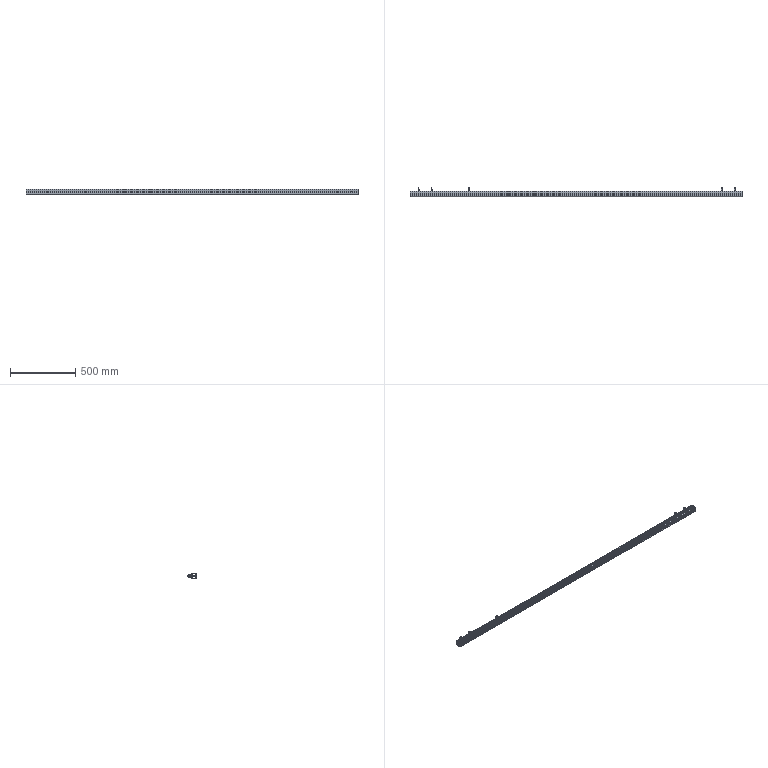Part | SolidWorks | features ReferencePattern 4, LocalLPattern 3 | 11 solids | 569 faces | box 2550 x 69.8 x 40 mm | volume 1229984 mm3 | plane 429 | cylinder 140 | commonest cylinder face diameters 3.2 x40 2.5 x30 3.8 x20 4 x20 6.5 x10 2 x5